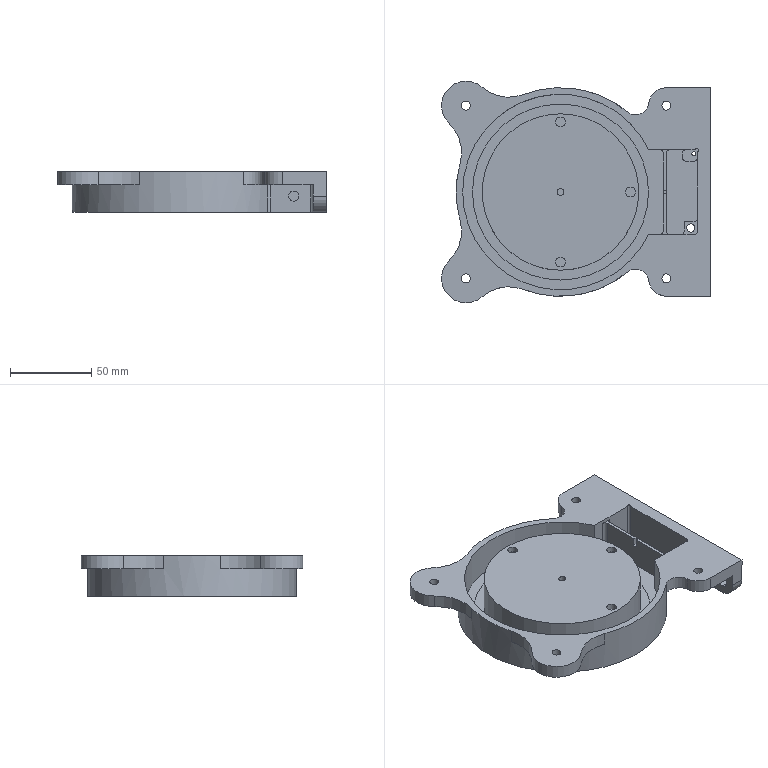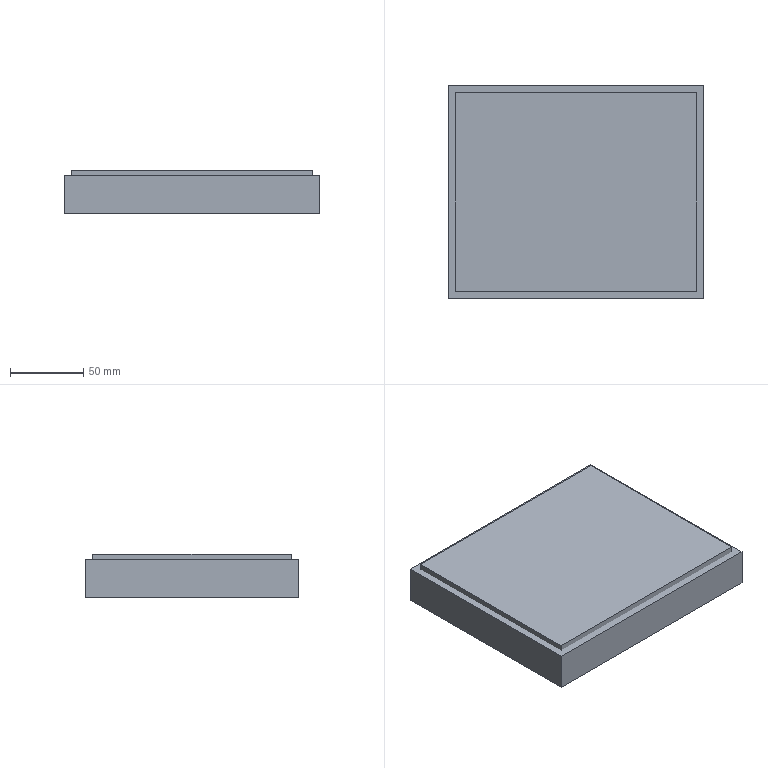CAM job | NX | 3-axis milling, drilling | part box 165 x 136 x 25 mm | stock box 175 x 146 x 30 mm
Tools:
number,name,description,diameter,corner_radius,flute_length,length,flutes
8,D80,Milling Tool-5 Parameters,80.0,0.0,50.0,75.0,2
7,D6A45,Milling Tool-5 Parameters,6.0,0.0,50.0,75.0,2
14,4.2ZT,Drilling Tool,4.2,0.0,35.0,50.0,2
12,2.0ZT,Drilling Tool,2.0,0.0,35.0,50.0,2
15,M5,Milling Tool-5 Parameters,5.0,0.0,30.0,30.0,4
10,D10,Milling Tool-5 Parameters,10.0,0.0,50.0,75.0,2
4,D4,Milling Tool-5 Parameters,4.0,0.0,50.0,75.0,2
2,D2,Milling Tool-5 Parameters,2.0,0.0,50.0,75.0,2
3,D3,Milling Tool-5 Parameters,3.0,0.0,50.0,75.0,2
11,D1.5,Milling Tool-5 Parameters,1.5,0.0,50.0,75.0,2
9,D10JING,Milling Tool-5 Parameters,10.0,0.0,50.0,75.0,2
1,D63,Milling Tool-5 Parameters,63.0,0.0,50.0,75.0,2
Operations:
program,operation,operation_type,tool,method,geometry_group,spindle_rpm,surface_speed,feed_per_tooth,feed_cut,feed_plunge,cut_length_mm,path_length_mm,cut_time_min,machine_time_min
1,FLOOR_WALL,VolumeBased25DMillingOperation,D63,METHOD,A,6500.0,1286.0,0.0962,1250.0,100.0,1084.797,1138.797,0.8678,0.8732
1,DRILLING,Operation,D6A45,METHOD,A,5000.0,94.0,0.025,250.0,0.0,36.0,597.492,0.144,0.2001
1,DRILLING_COPY,Operation,4.2ZT,METHOD,A,2000.0,26.0,0.0625,250.0,0.0,68.047,582.728,0.2722,0.3237
1,DRILLING_COPY_COPY_1,Operation,2.0ZT,METHOD,A,2000.0,12.0,0.03,120.0,0.0,27.101,114.202,0.2258,0.2346
1,DRILLING_COPY_COPY,Operation,M5,METHOD,A,300.0,4.0,0.0007,0.8,0.0,51.0,548.633,63.75,63.8
1,ADAPTIVE_MILLING,CavityMilling,D10,METHOD,A,9500.0,298.0,0.1316,2500.0,1000.0,19678.268,20775.094,7.88,7.99
1,CAVITY_MILL,CavityMilling,D10,METHOD,A,9500.0,298.0,0.1579,3000.0,1000.0,19660.724,20031.569,6.614,6.651
1,FLOOR_WALL_1,VolumeBased25DMillingOperation,D10JING,METHOD,A,9500.0,298.0,0.0658,1250.0,100.0,1784.325,2325.428,1.427,1.483
1,ZLEVEL_PROFILE,ZLevelMilling,D10JING,METHOD,A,9500.0,298.0,0.0658,1250.0,100.0,659.711,767.711,0.5278,0.5386
1,ZLEVEL_PROFILE_COPY,ZLevelMilling,D10JING,METHOD,A,9500.0,298.0,0.0658,1250.0,100.0,658.765,766.765,0.527,0.5378
1,CAVITY_MILL_COPY,CavityMilling,D4,METHOD,A,9500.0,119.0,0.0789,1500.0,1000.0,4289.653,6311.381,3.168,3.37
1,HOLE_MILLING,CylinderMilling,D3,METHOD,A,9500.0,89.0,0.0658,1250.0,100.0,391.743,702.365,0.3134,0.3445
1,PLANAR_PROFILE,PlanarMilling,D2,METHOD,A,9500.0,59.0,0.0658,1250.0,100.0,800.0,868.0,0.64,0.6468
1,PLANAR_MILL,PlanarMilling,D6A45,METHOD,A,9500.0,179.0,0.0658,1250.0,100.0,1470.933,2639.156,1.177,1.294
1,刀补,CylinderMilling,D3,METHOD,A,9500.0,89.0,0.0526,1000.0,100.0,151.08,461.703,0.1511,0.1821
2,FLOOR_WALL_COPY,VolumeBased25DMillingOperation,D80,METHOD,B,6500.0,1286.0,0.0962,1250.0,100.0,8549.97,11522.394,6.84,7.137
2,FACE_MILLING,FaceMilling,D80,METHOD,B,6500.0,1633.0,0.0962,1250.0,100.0,322.0,376.0,0.2576,0.263
2,PLANAR_MILL_1,PlanarMilling,D80,METHOD,B,6500.0,1633.0,0.0962,1250.0,100.0,704.0,1189.115,0.5632,0.6117
2,FLOOR_WALL_2,VolumeBased25DMillingOperation,D10,METHOD,B,9500.0,298.0,0.1316,2500.0,1000.0,20282.662,21967.05,8.262,8.43
2,FLOOR_WALL_1_COPY,VolumeBased25DMillingOperation,D10,METHOD,B,9500.0,298.0,0.0658,1250.0,100.0,1439.51,2220.092,1.152,1.233
2,ZLEVEL_PROFILE_1,ZLevelMilling,D10,METHOD,B,9500.0,298.0,0.1053,2000.0,1000.0,1335.563,1396.563,0.6917,0.6978
2,CAVITY_MILL_COPY_COPY,CavityMilling,D4,METHOD,B,9500.0,119.0,0.0789,1500.0,1000.0,1600.484,2949.249,1.204,1.339
2,HOLE_MILLING_1,CylinderMilling,D3,METHOD,B,9500.0,89.0,0.0658,1250.0,100.0,112.547,176.747,0.09,0.0965
2,HOLE_MILLING_COPY,CylinderMilling,D1.5,METHOD,B,9500.0,89.0,0.0658,1250.0,100.0,39.666,100.666,0.0317,0.0378
2,PLANAR_MILL_COPY,PlanarMilling,D6A45,METHOD,B,9500.0,179.0,0.0658,1250.0,100.0,966.227,1279.638,0.773,0.8043
2,PLANAR_MILL_COPY_COPY,PlanarMilling,D6A45,METHOD,B,9500.0,179.0,0.0658,1250.0,100.0,343.706,1758.793,0.275,0.4165
2,刀补3,CylinderMilling,D3,METHOD,B,9500.0,89.0,0.0658,1250.0,100.0,42.531,106.731,0.034,0.0404
2,刀补11,CylinderMilling,D1.5,METHOD,B,9500.0,89.0,0.0658,1250.0,100.0,10.76,71.76,0.0086,0.0147
2,刀补10,ZLevelMilling,D10,METHOD,B,9500.0,298.0,0.0658,1250.0,100.0,315.71,381.71,0.2526,0.2592